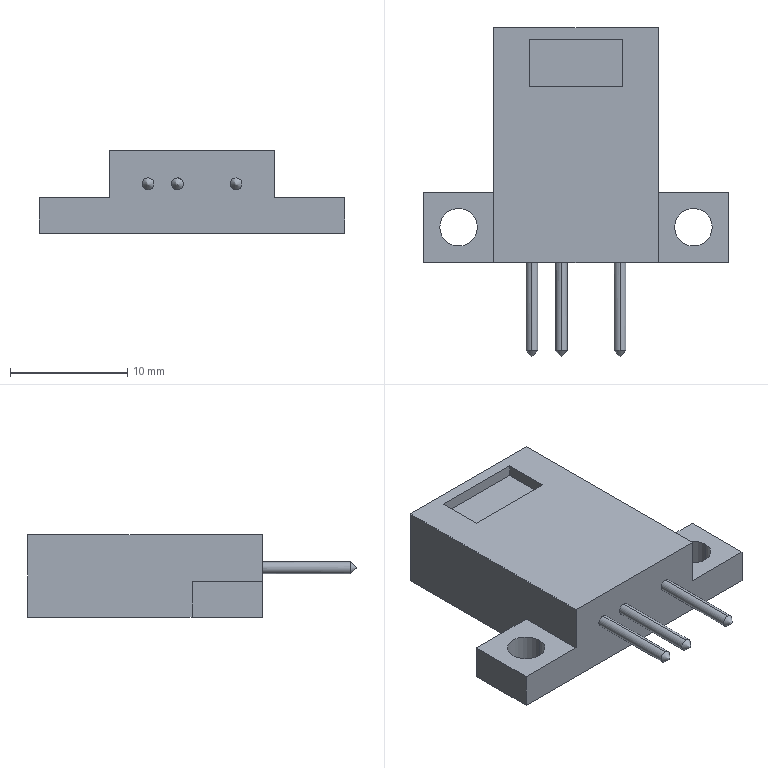Part | SolidWorks | features ICE 4, Dome 1, Extrusion 1 | 1 solid | 30 faces | box 26 x 27.999 x 7 mm | volume 2114 mm3 | plane 17 | cylinder 10 | spline 3 | commonest cylinder face diameters 1 x6 3.2 x4
STEP:
#1=CARTESIAN_POINT('',(3.75,-17.5,3.7));
#2=VERTEX_POINT('',#1);
#3=CARTESIAN_POINT('',(3.75,-17.5,4.7));
#4=VERTEX_POINT('',#3);
#5=CARTESIAN_POINT('',(3.75,-17.5,3.7));
#6=CARTESIAN_POINT('',(3.88,-17.5,3.7));
#7=CARTESIAN_POINT('',(4.011,-17.5,3.754));
#8=CARTESIAN_POINT('',(4.196,-17.5,3.938));
#9=CARTESIAN_POINT('',(4.25,-17.5,4.068));
#10=CARTESIAN_POINT('',(4.25,-17.5,4.332));
#11=CARTESIAN_POINT('',(4.196,-17.5,4.461));
#12=CARTESIAN_POINT('',(4.012,-17.5,4.646));
#13=CARTESIAN_POINT('',(3.882,-17.5,4.7));
#14=CARTESIAN_POINT('',(3.75,-17.5,4.7));
#15=B_SPLINE_CURVE_WITH_KNOTS('',3,(#5,#6,#7,#8,#9,#10,#11,#12,#13,#14),.UNSPECIFIED.,.F.,.F.,(4,2,2,2,4),(0.001565,0.001956,0.002347,0.002738,0.003129),.UNSPECIFIED.);
#16=EDGE_CURVE('',#2,#4,#15,.T.);
#17=ORIENTED_EDGE('',*,*,#16,.F.);
#18=CARTESIAN_POINT('',(3.75,-10.,3.7));
#19=VERTEX_POINT('',#18);
#20=CARTESIAN_POINT('',(3.75,-17.5,3.7));
#21=DIRECTION('',(0.,1.,0.));
#22=VECTOR('',#21,1000.);
#23=LINE('',#20,#22);
#24=EDGE_CURVE('',#2,#19,#23,.T.);
#25=ORIENTED_EDGE('',*,*,#24,.T.);
#26=CARTESIAN_POINT('',(3.75,-10.,4.7));
#27=VERTEX_POINT('',#26);
#28=CARTESIAN_POINT('',(3.75,-10.,4.2));
#29=DIRECTION('',(0.,-1.,0.));
#30=DIRECTION('',(0.,0.,1.));
#31=AXIS2_PLACEMENT_3D('',#28,#29,#30);
#32=CIRCLE('',#31,0.5);
#33=EDGE_CURVE('',#19,#27,#32,.T.);
#34=ORIENTED_EDGE('',*,*,#33,.T.);
#35=CARTESIAN_POINT('',(3.75,-17.5,4.7));
#36=DIRECTION('',(0.,1.,0.));
#37=VECTOR('',#36,1000.);
#38=LINE('',#35,#37);
#39=EDGE_CURVE('',#4,#27,#38,.T.);
#40=ORIENTED_EDGE('',*,*,#39,.F.);
#41=EDGE_LOOP('',(#17,#25,#34,#40));
#42=FACE_OUTER_BOUND('',#41,.T.);
#43=CARTESIAN_POINT('',(3.75,-17.5,4.2));
#44=DIRECTION('',(0.,1.,0.));
#45=DIRECTION('',(0.,0.,1.));
#46=AXIS2_PLACEMENT_3D('',#43,#44,#45);
#47=CYLINDRICAL_SURFACE('',#46,0.5);
#48=ADVANCED_FACE('',(#42),#47,.T.);
#49=CARTESIAN_POINT('',(-1.25,-17.5,3.7));
#50=VERTEX_POINT('',#49);
#51=CARTESIAN_POINT('',(-1.25,-17.5,4.7));
#52=VERTEX_POINT('',#51);
#53=CARTESIAN_POINT('',(-1.25,-17.5,3.7));
#54=CARTESIAN_POINT('',(-1.12,-17.5,3.7));
#55=CARTESIAN_POINT('',(-0.989,-17.5,3.754));
#56=CARTESIAN_POINT('',(-0.8044,-17.5,3.938));
#57=CARTESIAN_POINT('',(-0.7501,-17.5,4.068));
#58=CARTESIAN_POINT('',(-0.7499,-17.5,4.332));
#59=CARTESIAN_POINT('',(-0.804,-17.5,4.461));
#60=CARTESIAN_POINT('',(-0.9884,-17.5,4.646));
#61=CARTESIAN_POINT('',(-1.118,-17.5,4.7));
#62=CARTESIAN_POINT('',(-1.25,-17.5,4.7));
#63=B_SPLINE_CURVE_WITH_KNOTS('',3,(#53,#54,#55,#56,#57,#58,#59,#60,#61,#62),.UNSPECIFIED.,.F.,.F.,(4,2,2,2,4),(0.001565,0.001956,0.002347,0.002738,0.003129),.UNSPECIFIED.);
#64=EDGE_CURVE('',#50,#52,#63,.T.);
#65=ORIENTED_EDGE('',*,*,#64,.F.);
#66=CARTESIAN_POINT('',(-1.25,-10.,3.7));
#67=VERTEX_POINT('',#66);
#68=CARTESIAN_POINT('',(-1.25,-17.5,3.7));
#69=DIRECTION('',(0.,1.,0.));
#70=VECTOR('',#69,1000.);
#71=LINE('',#68,#70);
#72=EDGE_CURVE('',#50,#67,#71,.T.);
#73=ORIENTED_EDGE('',*,*,#72,.T.);
#74=CARTESIAN_POINT('',(-1.25,-10.,4.7));
#75=VERTEX_POINT('',#74);
#76=CARTESIAN_POINT('',(-1.25,-10.,4.2));
#77=DIRECTION('',(0.,-1.,0.));
#78=DIRECTION('',(0.,0.,1.));
#79=AXIS2_PLACEMENT_3D('',#76,#77,#78);
#80=CIRCLE('',#79,0.5);
#81=EDGE_CURVE('',#67,#75,#80,.T.);
#82=ORIENTED_EDGE('',*,*,#81,.T.);
#83=CARTESIAN_POINT('',(-1.25,-17.5,4.7));
#84=DIRECTION('',(0.,1.,0.));
#85=VECTOR('',#84,1000.);
#86=LINE('',#83,#85);
#87=EDGE_CURVE('',#52,#75,#86,.T.);
#88=ORIENTED_EDGE('',*,*,#87,.F.);
#89=EDGE_LOOP('',(#65,#73,#82,#88));
#90=FACE_OUTER_BOUND('',#89,.T.);
#91=CARTESIAN_POINT('',(-1.25,-17.5,4.2));
#92=DIRECTION('',(0.,1.,0.));
#93=DIRECTION('',(0.,0.,1.));
#94=AXIS2_PLACEMENT_3D('',#91,#92,#93);
#95=CYLINDRICAL_SURFACE('',#94,0.5);
#96=ADVANCED_FACE('',(#90),#95,.T.);
#97=CARTESIAN_POINT('',(-3.75,-17.5,3.7));
#98=VERTEX_POINT('',#97);
#99=CARTESIAN_POINT('',(-3.75,-17.5,4.7));
#100=VERTEX_POINT('',#99);
#101=CARTESIAN_POINT('',(-3.75,-17.5,3.7));
#102=CARTESIAN_POINT('',(-3.62,-17.5,3.7));
#103=CARTESIAN_POINT('',(-3.489,-17.5,3.754));
#104=CARTESIAN_POINT('',(-3.304,-17.5,3.938));
#105=CARTESIAN_POINT('',(-3.25,-17.5,4.068));
#106=CARTESIAN_POINT('',(-3.25,-17.5,4.332));
#107=CARTESIAN_POINT('',(-3.304,-17.5,4.461));
#108=CARTESIAN_POINT('',(-3.488,-17.5,4.646));
#109=CARTESIAN_POINT('',(-3.618,-17.5,4.7));
#110=CARTESIAN_POINT('',(-3.75,-17.5,4.7));
#111=B_SPLINE_CURVE_WITH_KNOTS('',3,(#101,#102,#103,#104,#105,#106,#107,#108,#109,#110),.UNSPECIFIED.,.F.,.F.,(4,2,2,2,4),(0.001565,0.001956,0.002347,0.002738,0.003129),.UNSPECIFIED.);
#112=EDGE_CURVE('',#98,#100,#111,.T.);
#113=ORIENTED_EDGE('',*,*,#112,.F.);
#114=CARTESIAN_POINT('',(-3.75,-10.,3.7));
#115=VERTEX_POINT('',#114);
#116=CARTESIAN_POINT('',(-3.75,-17.5,3.7));
#117=DIRECTION('',(0.,1.,0.));
#118=VECTOR('',#117,1000.);
#119=LINE('',#116,#118);
#120=EDGE_CURVE('',#98,#115,#119,.T.);
#121=ORIENTED_EDGE('',*,*,#120,.T.);
#122=CARTESIAN_POINT('',(-3.75,-10.,4.7));
#123=VERTEX_POINT('',#122);
#124=CARTESIAN_POINT('',(-3.75,-10.,4.2));
#125=DIRECTION('',(0.,-1.,0.));
#126=DIRECTION('',(0.,0.,1.));
#127=AXIS2_PLACEMENT_3D('',#124,#125,#126);
#128=CIRCLE('',#127,0.5);
#129=EDGE_CURVE('',#115,#123,#128,.T.);
#130=ORIENTED_EDGE('',*,*,#129,.T.);
#131=CARTESIAN_POINT('',(-3.75,-17.5,4.7));
#132=DIRECTION('',(0.,1.,0.));
#133=VECTOR('',#132,1000.);
#134=LINE('',#131,#133);
#135=EDGE_CURVE('',#100,#123,#134,.T.);
#136=ORIENTED_EDGE('',*,*,#135,.F.);
#137=EDGE_LOOP('',(#113,#121,#130,#136));
#138=FACE_OUTER_BOUND('',#137,.T.);
#139=CARTESIAN_POINT('',(-3.75,-17.5,4.2));
#140=DIRECTION('',(0.,1.,0.));
#141=DIRECTION('',(0.,0.,1.));
#142=AXIS2_PLACEMENT_3D('',#139,#140,#141);
#143=CYLINDRICAL_SURFACE('',#142,0.5);
#144=ADVANCED_FACE('',(#138),#143,.T.);
#145=CARTESIAN_POINT('',(8.4,-7.,0.));
#146=VERTEX_POINT('',#145);
#147=CARTESIAN_POINT('',(11.6,-7.,0.));
#148=VERTEX_POINT('',#147);
#149=CARTESIAN_POINT('',(10.,-7.,0.));
#150=DIRECTION('',(0.,0.,1.));
#151=DIRECTION('',(1.,0.,0.));
#152=AXIS2_PLACEMENT_3D('',#149,#150,#151);
#153=CIRCLE('',#152,1.6);
#154=EDGE_CURVE('',#146,#148,#153,.T.);
#155=ORIENTED_EDGE('',*,*,#154,.F.);
#156=CARTESIAN_POINT('',(8.4,-7.,3.));
#157=VERTEX_POINT('',#156);
#158=CARTESIAN_POINT('',(8.4,-7.,-0.00005));
#159=DIRECTION('',(0.,0.,1.));
#160=VECTOR('',#159,1000.);
#161=LINE('',#158,#160);
#162=EDGE_CURVE('',#146,#157,#161,.T.);
#163=ORIENTED_EDGE('',*,*,#162,.T.);
#164=CARTESIAN_POINT('',(11.6,-7.,3.));
#165=VERTEX_POINT('',#164);
#166=CARTESIAN_POINT('',(10.,-7.,3.));
#167=DIRECTION('',(0.,0.,1.));
#168=DIRECTION('',(-1.,0.,0.));
#169=AXIS2_PLACEMENT_3D('',#166,#167,#168);
#170=CIRCLE('',#169,1.6);
#171=EDGE_CURVE('',#157,#165,#170,.T.);
#172=ORIENTED_EDGE('',*,*,#171,.T.);
#173=CARTESIAN_POINT('',(11.6,-7.,-0.00005));
#174=DIRECTION('',(0.,0.,1.));
#175=VECTOR('',#174,1000.);
#176=LINE('',#173,#175);
#177=EDGE_CURVE('',#148,#165,#176,.T.);
#178=ORIENTED_EDGE('',*,*,#177,.F.);
#179=EDGE_LOOP('',(#155,#163,#172,#178));
#180=FACE_OUTER_BOUND('',#179,.T.);
#181=CARTESIAN_POINT('',(10.,-7.,-0.00005));
#182=DIRECTION('',(0.,0.,1.));
#183=DIRECTION('',(1.,0.,0.));
#184=AXIS2_PLACEMENT_3D('',#181,#182,#183);
#185=CYLINDRICAL_SURFACE('',#184,1.6);
#186=ADVANCED_FACE('',(#180),#185,.F.);
#187=CARTESIAN_POINT('',(-11.6,-7.,0.));
#188=VERTEX_POINT('',#187);
#189=CARTESIAN_POINT('',(-8.4,-7.,0.));
#190=VERTEX_POINT('',#189);
#191=CARTESIAN_POINT('',(-10.,-7.,0.));
#192=DIRECTION('',(0.,0.,1.));
#193=DIRECTION('',(1.,0.,0.));
#194=AXIS2_PLACEMENT_3D('',#191,#192,#193);
#195=CIRCLE('',#194,1.6);
#196=EDGE_CURVE('',#188,#190,#195,.T.);
#197=ORIENTED_EDGE('',*,*,#196,.F.);
#198=CARTESIAN_POINT('',(-11.6,-7.,3.));
#199=VERTEX_POINT('',#198);
#200=CARTESIAN_POINT('',(-11.6,-7.,-0.00005));
#201=DIRECTION('',(0.,0.,1.));
#202=VECTOR('',#201,1000.);
#203=LINE('',#200,#202);
#204=EDGE_CURVE('',#188,#199,#203,.T.);
#205=ORIENTED_EDGE('',*,*,#204,.T.);
#206=CARTESIAN_POINT('',(-8.4,-7.,3.));
#207=VERTEX_POINT('',#206);
#208=CARTESIAN_POINT('',(-10.,-7.,3.));
#209=DIRECTION('',(0.,0.,1.));
#210=DIRECTION('',(1.,0.,0.));
#211=AXIS2_PLACEMENT_3D('',#208,#209,#210);
#212=CIRCLE('',#211,1.6);
#213=EDGE_CURVE('',#199,#207,#212,.T.);
#214=ORIENTED_EDGE('',*,*,#213,.T.);
#215=CARTESIAN_POINT('',(-8.4,-7.,-0.00005));
#216=DIRECTION('',(0.,0.,1.));
#217=VECTOR('',#216,1000.);
#218=LINE('',#215,#217);
#219=EDGE_CURVE('',#190,#207,#218,.T.);
#220=ORIENTED_EDGE('',*,*,#219,.F.);
#221=EDGE_LOOP('',(#197,#205,#214,#220));
#222=FACE_OUTER_BOUND('',#221,.T.);
#223=CARTESIAN_POINT('',(-10.,-7.,-0.00005));
#224=DIRECTION('',(0.,0.,1.));
#225=DIRECTION('',(1.,0.,0.));
#226=AXIS2_PLACEMENT_3D('',#223,#224,#225);
#227=CYLINDRICAL_SURFACE('',#226,1.6);
#228=ADVANCED_FACE('',(#222),#227,.F.);
#229=CARTESIAN_POINT('',(-1.25,-10.,4.2));
#230=DIRECTION('',(0.,-1.,0.));
#231=DIRECTION('',(0.,0.,1.));
#232=AXIS2_PLACEMENT_3D('',#229,#230,#231);
#233=CIRCLE('',#232,0.5);
#234=EDGE_CURVE('',#75,#67,#233,.T.);
#235=ORIENTED_EDGE('',*,*,#234,.F.);
#236=ORIENTED_EDGE('',*,*,#81,.F.);
#237=EDGE_LOOP('',(#235,#236));
#238=FACE_BOUND('',#237,.T.);
#239=CARTESIAN_POINT('',(-13.,-10.,0.));
#240=VERTEX_POINT('',#239);
#241=CARTESIAN_POINT('',(13.,-10.,0.));
#242=VERTEX_POINT('',#241);
#243=CARTESIAN_POINT('',(-7.,-10.,0.));
#244=DIRECTION('',(1.,0.,0.));
#245=VECTOR('',#244,1000.);
#246=LINE('',#243,#245);
#247=EDGE_CURVE('',#240,#242,#246,.T.);
#248=ORIENTED_EDGE('',*,*,#247,.T.);
#249=CARTESIAN_POINT('',(13.,-10.,3.));
#250=VERTEX_POINT('',#249);
#251=CARTESIAN_POINT('',(13.,-10.,3.));
#252=DIRECTION('',(0.,0.,-1.));
#253=VECTOR('',#252,1000.);
#254=LINE('',#251,#253);
#255=EDGE_CURVE('',#250,#242,#254,.T.);
#256=ORIENTED_EDGE('',*,*,#255,.F.);
#257=CARTESIAN_POINT('',(7.,-10.,3.));
#258=VERTEX_POINT('',#257);
#259=CARTESIAN_POINT('',(7.,-10.,3.));
#260=DIRECTION('',(-1.,0.,0.));
#261=VECTOR('',#260,1000.);
#262=LINE('',#259,#261);
#263=EDGE_CURVE('',#250,#258,#262,.T.);
#264=ORIENTED_EDGE('',*,*,#263,.T.);
#265=CARTESIAN_POINT('',(7.,-10.,7.));
#266=VERTEX_POINT('',#265);
#267=CARTESIAN_POINT('',(7.,-10.,7.));
#268=DIRECTION('',(0.,0.,-1.));
#269=VECTOR('',#268,1000.);
#270=LINE('',#267,#269);
#271=EDGE_CURVE('',#266,#258,#270,.T.);
#272=ORIENTED_EDGE('',*,*,#271,.F.);
#273=CARTESIAN_POINT('',(-7.,-10.,7.));
#274=VERTEX_POINT('',#273);
#275=CARTESIAN_POINT('',(-7.,-10.,7.));
#276=DIRECTION('',(1.,0.,0.));
#277=VECTOR('',#276,1000.);
#278=LINE('',#275,#277);
#279=EDGE_CURVE('',#274,#266,#278,.T.);
#280=ORIENTED_EDGE('',*,*,#279,.F.);
#281=CARTESIAN_POINT('',(-7.,-10.,3.));
#282=VERTEX_POINT('',#281);
#283=CARTESIAN_POINT('',(-7.,-10.,7.));
#284=DIRECTION('',(0.,0.,-1.));
#285=VECTOR('',#284,1000.);
#286=LINE('',#283,#285);
#287=EDGE_CURVE('',#274,#282,#286,.T.);
#288=ORIENTED_EDGE('',*,*,#287,.T.);
#289=CARTESIAN_POINT('',(-13.,-10.,3.));
#290=VERTEX_POINT('',#289);
#291=CARTESIAN_POINT('',(-7.,-10.,3.));
#292=DIRECTION('',(-1.,0.,0.));
#293=VECTOR('',#292,1000.);
#294=LINE('',#291,#293);
#295=EDGE_CURVE('',#282,#290,#294,.T.);
#296=ORIENTED_EDGE('',*,*,#295,.T.);
#297=CARTESIAN_POINT('',(-13.,-10.,3.));
#298=DIRECTION('',(0.,0.,-1.));
#299=VECTOR('',#298,1000.);
#300=LINE('',#297,#299);
#301=EDGE_CURVE('',#290,#240,#300,.T.);
#302=ORIENTED_EDGE('',*,*,#301,.T.);
#303=EDGE_LOOP('',(#248,#256,#264,#272,#280,#288,#296,#302));
#304=FACE_OUTER_BOUND('',#303,.T.);
#305=CARTESIAN_POINT('',(-3.75,-10.,4.2));
#306=DIRECTION('',(0.,-1.,0.));
#307=DIRECTION('',(0.,0.,1.));
#308=AXIS2_PLACEMENT_3D('',#305,#306,#307);
#309=CIRCLE('',#308,0.5);
#310=EDGE_CURVE('',#123,#115,#309,.T.);
#311=ORIENTED_EDGE('',*,*,#310,.F.);
#312=ORIENTED_EDGE('',*,*,#129,.F.);
#313=EDGE_LOOP('',(#311,#312));
#314=FACE_BOUND('',#313,.T.);
#315=CARTESIAN_POINT('',(3.75,-10.,4.2));
#316=DIRECTION('',(0.,-1.,0.));
#317=DIRECTION('',(0.,0.,1.));
#318=AXIS2_PLACEMENT_3D('',#315,#316,#317);
#319=CIRCLE('',#318,0.5);
#320=EDGE_CURVE('',#27,#19,#319,.T.);
#321=ORIENTED_EDGE('',*,*,#320,.F.);
#322=ORIENTED_EDGE('',*,*,#33,.F.);
#323=EDGE_LOOP('',(#321,#322));
#324=FACE_BOUND('',#323,.T.);
#325=CARTESIAN_POINT('',(-7.,-10.,7.));
#326=DIRECTION('',(0.,1.,0.));
#327=DIRECTION('',(0.,0.,1.));
#328=AXIS2_PLACEMENT_3D('',#325,#326,#327);
#329=PLANE('',#328);
#330=ADVANCED_FACE('',(#238,#304,#314,#324),#329,.F.);
#331=CARTESIAN_POINT('',(-7.,-4.,3.));
#332=VERTEX_POINT('',#331);
#333=CARTESIAN_POINT('',(-7.,-4.,0.));
#334=VERTEX_POINT('',#333);
#335=CARTESIAN_POINT('',(-7.,-4.,3.));
#336=DIRECTION('',(0.,0.,-1.));
#337=VECTOR('',#336,1000.);
#338=LINE('',#335,#337);
#339=EDGE_CURVE('',#332,#334,#338,.T.);
#340=ORIENTED_EDGE('',*,*,#339,.F.);
#341=CARTESIAN_POINT('',(-7.,-4.,3.));
#342=DIRECTION('',(0.,-1.,0.));
#343=VECTOR('',#342,1000.);
#344=LINE('',#341,#343);
#345=EDGE_CURVE('',#332,#282,#344,.T.);
#346=ORIENTED_EDGE('',*,*,#345,.T.);
#347=ORIENTED_EDGE('',*,*,#287,.F.);
#348=CARTESIAN_POINT('',(-7.,10.,7.));
#349=VERTEX_POINT('',#348);
#350=CARTESIAN_POINT('',(-7.,10.,7.));
#351=DIRECTION('',(0.,-1.,0.));
#352=VECTOR('',#351,1000.);
#353=LINE('',#350,#352);
#354=EDGE_CURVE('',#349,#274,#353,.T.);
#355=ORIENTED_EDGE('',*,*,#354,.F.);
#356=CARTESIAN_POINT('',(-7.,10.,0.));
#357=VERTEX_POINT('',#356);
#358=CARTESIAN_POINT('',(-7.,10.,7.));
#359=DIRECTION('',(0.,0.,-1.));
#360=VECTOR('',#359,1000.);
#361=LINE('',#358,#360);
#362=EDGE_CURVE('',#349,#357,#361,.T.);
#363=ORIENTED_EDGE('',*,*,#362,.T.);
#364=CARTESIAN_POINT('',(-7.,10.,0.));
#365=DIRECTION('',(0.,-1.,0.));
#366=VECTOR('',#365,1000.);
#367=LINE('',#364,#366);
#368=EDGE_CURVE('',#357,#334,#367,.T.);
#369=ORIENTED_EDGE('',*,*,#368,.T.);
#370=EDGE_LOOP('',(#340,#346,#347,#355,#363,#369));
#371=FACE_OUTER_BOUND('',#370,.T.);
#372=CARTESIAN_POINT('',(-7.,10.,7.));
#373=DIRECTION('',(1.,0.,0.));
#374=DIRECTION('',(0.,1.,0.));
#375=AXIS2_PLACEMENT_3D('',#372,#373,#374);
#376=PLANE('',#375);
#377=ADVANCED_FACE('',(#371),#376,.F.);
#378=ORIENTED_EDGE('',*,*,#271,.T.);
#379=CARTESIAN_POINT('',(7.,-4.,3.));
#380=VERTEX_POINT('',#379);
#381=CARTESIAN_POINT('',(7.,-4.,3.));
#382=DIRECTION('',(0.,1.,0.));
#383=VECTOR('',#382,1000.);
#384=LINE('',#381,#383);
#385=EDGE_CURVE('',#258,#380,#384,.T.);
#386=ORIENTED_EDGE('',*,*,#385,.T.);
#387=CARTESIAN_POINT('',(7.,-4.,0.));
#388=VERTEX_POINT('',#387);
#389=CARTESIAN_POINT('',(7.,-4.,3.));
#390=DIRECTION('',(0.,0.,-1.));
#391=VECTOR('',#390,1000.);
#392=LINE('',#389,#391);
#393=EDGE_CURVE('',#380,#388,#392,.T.);
#394=ORIENTED_EDGE('',*,*,#393,.T.);
#395=CARTESIAN_POINT('',(7.,10.,0.));
#396=VERTEX_POINT('',#395);
#397=CARTESIAN_POINT('',(7.,10.,0.));
#398=DIRECTION('',(0.,1.,0.));
#399=VECTOR('',#398,1000.);
#400=LINE('',#397,#399);
#401=EDGE_CURVE('',#388,#396,#400,.T.);
#402=ORIENTED_EDGE('',*,*,#401,.T.);
#403=CARTESIAN_POINT('',(7.,10.,7.));
#404=VERTEX_POINT('',#403);
#405=CARTESIAN_POINT('',(7.,10.,7.));
#406=DIRECTION('',(0.,0.,-1.));
#407=VECTOR('',#406,1000.);
#408=LINE('',#405,#407);
#409=EDGE_CURVE('',#404,#396,#408,.T.);
#410=ORIENTED_EDGE('',*,*,#409,.F.);
#411=CARTESIAN_POINT('',(7.,10.,7.));
#412=DIRECTION('',(0.,1.,0.));
#413=VECTOR('',#412,1000.);
#414=LINE('',#411,#413);
#415=EDGE_CURVE('',#266,#404,#414,.T.);
#416=ORIENTED_EDGE('',*,*,#415,.F.);
#417=EDGE_LOOP('',(#378,#386,#394,#402,#410,#416));
#418=FACE_OUTER_BOUND('',#417,.T.);
#419=CARTESIAN_POINT('',(7.,10.,7.));
#420=DIRECTION('',(-1.,0.,0.));
#421=DIRECTION('',(0.,-1.,0.));
#422=AXIS2_PLACEMENT_3D('',#419,#420,#421);
#423=PLANE('',#422);
#424=ADVANCED_FACE('',(#418),#423,.F.);
#425=CARTESIAN_POINT('',(-7.,10.,0.));
#426=DIRECTION('',(-1.,0.,0.));
#427=VECTOR('',#426,1000.);
#428=LINE('',#425,#427);
#429=EDGE_CURVE('',#396,#357,#428,.T.);
#430=ORIENTED_EDGE('',*,*,#429,.T.);
#431=ORIENTED_EDGE('',*,*,#362,.F.);
#432=CARTESIAN_POINT('',(-7.,10.,7.));
#433=DIRECTION('',(-1.,0.,0.));
#434=VECTOR('',#433,1000.);
#435=LINE('',#432,#434);
#436=EDGE_CURVE('',#404,#349,#435,.T.);
#437=ORIENTED_EDGE('',*,*,#436,.F.);
#438=ORIENTED_EDGE('',*,*,#409,.T.);
#439=EDGE_LOOP('',(#430,#431,#437,#438));
#440=FACE_OUTER_BOUND('',#439,.T.);
#441=CARTESIAN_POINT('',(-7.,10.,7.));
#442=DIRECTION('',(0.,-1.,0.));
#443=DIRECTION('',(0.,0.,-1.));
#444=AXIS2_PLACEMENT_3D('',#441,#442,#443);
#445=PLANE('',#444);
#446=ADVANCED_FACE('',(#440),#445,.F.);
#447=CARTESIAN_POINT('',(-4.,9.,7.));
#448=VERTEX_POINT('',#447);
#449=CARTESIAN_POINT('',(-4.,5.,7.));
#450=VERTEX_POINT('',#449);
#451=CARTESIAN_POINT('',(-4.,9.,7.));
#452=DIRECTION('',(0.,-1.,0.));
#453=VECTOR('',#452,1000.);
#454=LINE('',#451,#453);
#455=EDGE_CURVE('',#448,#450,#454,.T.);
#456=ORIENTED_EDGE('',*,*,#455,.F.);
#457=CARTESIAN_POINT('',(4.,9.,7.));
#458=VERTEX_POINT('',#457);
#459=CARTESIAN_POINT('',(-4.,9.,7.));
#460=DIRECTION('',(-1.,0.,0.));
#461=VECTOR('',#460,1000.);
#462=LINE('',#459,#461);
#463=EDGE_CURVE('',#458,#448,#462,.T.);
#464=ORIENTED_EDGE('',*,*,#463,.F.);
#465=CARTESIAN_POINT('',(4.,5.,7.));
#466=VERTEX_POINT('',#465);
#467=CARTESIAN_POINT('',(4.,9.,7.));
#468=DIRECTION('',(0.,1.,0.));
#469=VECTOR('',#468,1000.);
#470=LINE('',#467,#469);
#471=EDGE_CURVE('',#466,#458,#470,.T.);
#472=ORIENTED_EDGE('',*,*,#471,.F.);
#473=CARTESIAN_POINT('',(-4.,5.,7.));
#474=DIRECTION('',(1.,0.,0.));
#475=VECTOR('',#474,1000.);
#476=LINE('',#473,#475);
#477=EDGE_CURVE('',#450,#466,#476,.T.);
#478=ORIENTED_EDGE('',*,*,#477,.F.);
#479=EDGE_LOOP('',(#456,#464,#472,#478));
#480=FACE_BOUND('',#479,.T.);
#481=ORIENTED_EDGE('',*,*,#354,.T.);
#482=ORIENTED_EDGE('',*,*,#279,.T.);
#483=ORIENTED_EDGE('',*,*,#415,.T.);
#484=ORIENTED_EDGE('',*,*,#436,.T.);
#485=EDGE_LOOP('',(#481,#482,#483,#484));
#486=FACE_OUTER_BOUND('',#485,.T.);
#487=CARTESIAN_POINT('',(-7.,-10.,7.));
#488=DIRECTION('',(0.,0.,1.));
#489=DIRECTION('',(1.,0.,0.));
#490=AXIS2_PLACEMENT_3D('',#487,#488,#489);
#491=PLANE('',#490);
#492=ADVANCED_FACE('',(#480,#486),#491,.T.);
#493=CARTESIAN_POINT('',(10.,-7.,0.));
#494=DIRECTION('',(0.,0.,1.));
#495=DIRECTION('',(1.,0.,0.));
#496=AXIS2_PLACEMENT_3D('',#493,#494,#495);
#497=CIRCLE('',#496,1.6);
#498=EDGE_CURVE('',#148,#146,#497,.T.);
#499=ORIENTED_EDGE('',*,*,#498,.T.);
#500=ORIENTED_EDGE('',*,*,#154,.T.);
#501=EDGE_LOOP('',(#499,#500));
#502=FACE_BOUND('',#501,.T.);
#503=CARTESIAN_POINT('',(-10.,-7.,0.));
#504=DIRECTION('',(0.,0.,1.));
#505=DIRECTION('',(1.,0.,0.));
#506=AXIS2_PLACEMENT_3D('',#503,#504,#505);
#507=CIRCLE('',#506,1.6);
#508=EDGE_CURVE('',#190,#188,#507,.T.);
#509=ORIENTED_EDGE('',*,*,#508,.T.);
#510=ORIENTED_EDGE('',*,*,#196,.T.);
#511=EDGE_LOOP('',(#509,#510));
#512=FACE_BOUND('',#511,.T.);
#513=ORIENTED_EDGE('',*,*,#368,.F.);
#514=ORIENTED_EDGE('',*,*,#429,.F.);
#515=ORIENTED_EDGE('',*,*,#401,.F.);
#516=CARTESIAN_POINT('',(13.,-4.,0.));
#517=VERTEX_POINT('',#516);
#518=CARTESIAN_POINT('',(7.,-4.,0.));
#519=DIRECTION('',(1.,0.,0.));
#520=VECTOR('',#519,1000.);
#521=LINE('',#518,#520);
#522=EDGE_CURVE('',#388,#517,#521,.T.);
#523=ORIENTED_EDGE('',*,*,#522,.T.);
#524=CARTESIAN_POINT('',(13.,-4.,0.));
#525=DIRECTION('',(0.,-1.,0.));
#526=VECTOR('',#525,1000.);
#527=LINE('',#524,#526);
#528=EDGE_CURVE('',#517,#242,#527,.T.);
#529=ORIENTED_EDGE('',*,*,#528,.T.);
#530=ORIENTED_EDGE('',*,*,#247,.F.);
#531=CARTESIAN_POINT('',(-13.,-4.,0.));
#532=VERTEX_POINT('',#531);
#533=CARTESIAN_POINT('',(-13.,-4.,0.));
#534=DIRECTION('',(0.,1.,0.));
#535=VECTOR('',#534,1000.);
#536=LINE('',#533,#535);
#537=EDGE_CURVE('',#240,#532,#536,.T.);
#538=ORIENTED_EDGE('',*,*,#537,.T.);
#539=CARTESIAN_POINT('',(-7.,-4.,0.));
#540=DIRECTION('',(1.,0.,0.));
#541=VECTOR('',#540,1000.);
#542=LINE('',#539,#541);
#543=EDGE_CURVE('',#532,#334,#542,.T.);
#544=ORIENTED_EDGE('',*,*,#543,.T.);
#545=EDGE_LOOP('',(#513,#514,#515,#523,#529,#530,#538,#544));
#546=FACE_OUTER_BOUND('',#545,.T.);
#547=CARTESIAN_POINT('',(-7.,-10.,0.));
#548=DIRECTION('',(0.,0.,1.));
#549=DIRECTION('',(1.,0.,0.));
#550=AXIS2_PLACEMENT_3D('',#547,#548,#549);
#551=PLANE('',#550);
#552=ADVANCED_FACE('',(#502,#512,#546),#551,.F.);
#553=ORIENTED_EDGE('',*,*,#528,.F.);
#554=CARTESIAN_POINT('',(13.,-4.,3.));
#555=VERTEX_POINT('',#554);
#556=CARTESIAN_POINT('',(13.,-4.,3.));
#557=DIRECTION('',(0.,0.,-1.));
#558=VECTOR('',#557,1000.);
#559=LINE('',#556,#558);
#560=EDGE_CURVE('',#555,#517,#559,.T.);
#561=ORIENTED_EDGE('',*,*,#560,.F.);
#562=CARTESIAN_POINT('',(13.,-4.,3.));
#563=DIRECTION('',(0.,-1.,0.));
#564=VECTOR('',#563,1000.);
#565=LINE('',#562,#564);
#566=EDGE_CURVE('',#555,#250,#565,.T.);
#567=ORIENTED_EDGE('',*,*,#566,.T.);
#568=ORIENTED_EDGE('',*,*,#255,.T.);
#569=EDGE_LOOP('',(#553,#561,#567,#568));
#570=FACE_OUTER_BOUND('',#569,.T.);
#571=CARTESIAN_POINT('',(13.,-4.,3.));
#572=DIRECTION('',(1.,0.,0.));
#573=DIRECTION('',(0.,1.,0.));
#574=AXIS2_PLACEMENT_3D('',#571,#572,#573);
#575=PLANE('',#574);
#576=ADVANCED_FACE('',(#570),#575,.T.);
#577=ORIENTED_EDGE('',*,*,#522,.F.);
#578=ORIENTED_EDGE('',*,*,#393,.F.);
#579=CARTESIAN_POINT('',(7.,-4.,3.));
#580=DIRECTION('',(1.,0.,0.));
#581=VECTOR('',#580,1000.);
#582=LINE('',#579,#581);
#583=EDGE_CURVE('',#380,#555,#582,.T.);
#584=ORIENTED_EDGE('',*,*,#583,.T.);
#585=ORIENTED_EDGE('',*,*,#560,.T.);
#586=EDGE_LOOP('',(#577,#578,#584,#585));
#587=FACE_OUTER_BOUND('',#586,.T.);
#588=CARTESIAN_POINT('',(7.,-4.,3.));
#589=DIRECTION('',(0.,1.,0.));
#590=DIRECTION('',(-1.,0.,0.));
#591=AXIS2_PLACEMENT_3D('',#588,#589,#590);
#592=PLANE('',#591);
#593=ADVANCED_FACE('',(#587),#592,.T.);
#594=CARTESIAN_POINT('',(10.,-7.,3.));
#595=DIRECTION('',(0.,0.,1.));
#596=DIRECTION('',(-1.,0.,0.));
#597=AXIS2_PLACEMENT_3D('',#594,#595,#596);
#598=CIRCLE('',#597,1.6);
#599=EDGE_CURVE('',#165,#157,#598,.T.);
#600=ORIENTED_EDGE('',*,*,#599,.F.);
#601=ORIENTED_EDGE('',*,*,#171,.F.);
#602=EDGE_LOOP('',(#600,#601));
#603=FACE_BOUND('',#602,.T.);
#604=ORIENTED_EDGE('',*,*,#385,.F.);
#605=ORIENTED_EDGE('',*,*,#263,.F.);
#606=ORIENTED_EDGE('',*,*,#566,.F.);
#607=ORIENTED_EDGE('',*,*,#583,.F.);
#608=EDGE_LOOP('',(#604,#605,#606,#607));
#609=FACE_OUTER_BOUND('',#608,.T.);
#610=CARTESIAN_POINT('',(7.,-10.,3.));
#611=DIRECTION('',(0.,0.,1.));
#612=DIRECTION('',(1.,0.,0.));
#613=AXIS2_PLACEMENT_3D('',#610,#611,#612);
#614=PLANE('',#613);
#615=ADVANCED_FACE('',(#603,#609),#614,.T.);
#616=ORIENTED_EDGE('',*,*,#543,.F.);
#617=CARTESIAN_POINT('',(-13.,-4.,3.));
#618=VERTEX_POINT('',#617);
#619=CARTESIAN_POINT('',(-13.,-4.,3.));
#620=DIRECTION('',(0.,0.,-1.));
#621=VECTOR('',#620,1000.);
#622=LINE('',#619,#621);
#623=EDGE_CURVE('',#618,#532,#622,.T.);
#624=ORIENTED_EDGE('',*,*,#623,.F.);
#625=CARTESIAN_POINT('',(-7.,-4.,3.));
#626=DIRECTION('',(1.,0.,0.));
#627=VECTOR('',#626,1000.);
#628=LINE('',#625,#627);
#629=EDGE_CURVE('',#618,#332,#628,.T.);
#630=ORIENTED_EDGE('',*,*,#629,.T.);
#631=ORIENTED_EDGE('',*,*,#339,.T.);
#632=EDGE_LOOP('',(#616,#624,#630,#631));
#633=FACE_OUTER_BOUND('',#632,.T.);
#634=CARTESIAN_POINT('',(-7.,-4.,3.));
#635=DIRECTION('',(0.,1.,0.));
#636=DIRECTION('',(-1.,0.,0.));
#637=AXIS2_PLACEMENT_3D('',#634,#635,#636);
#638=PLANE('',#637);
#639=ADVANCED_FACE('',(#633),#638,.T.);
#640=ORIENTED_EDGE('',*,*,#537,.F.);
#641=ORIENTED_EDGE('',*,*,#301,.F.);
#642=CARTESIAN_POINT('',(-13.,-4.,3.));
#643=DIRECTION('',(0.,1.,0.));
#644=VECTOR('',#643,1000.);
#645=LINE('',#642,#644);
#646=EDGE_CURVE('',#290,#618,#645,.T.);
#647=ORIENTED_EDGE('',*,*,#646,.T.);
#648=ORIENTED_EDGE('',*,*,#623,.T.);
#649=EDGE_LOOP('',(#640,#641,#647,#648));
#650=FACE_OUTER_BOUND('',#649,.T.);
#651=CARTESIAN_POINT('',(-13.,-4.,3.));
#652=DIRECTION('',(-1.,0.,0.));
#653=DIRECTION('',(0.,0.,1.));
#654=AXIS2_PLACEMENT_3D('',#651,#652,#653);
#655=PLANE('',#654);
#656=ADVANCED_FACE('',(#650),#655,.T.);
#657=CARTESIAN_POINT('',(-10.,-7.,3.));
#658=DIRECTION('',(0.,0.,1.));
#659=DIRECTION('',(1.,0.,0.));
#660=AXIS2_PLACEMENT_3D('',#657,#658,#659);
#661=CIRCLE('',#660,1.6);
#662=EDGE_CURVE('',#207,#199,#661,.T.);
#663=ORIENTED_EDGE('',*,*,#662,.F.);
#664=ORIENTED_EDGE('',*,*,#213,.F.);
#665=EDGE_LOOP('',(#663,#664));
#666=FACE_BOUND('',#665,.T.);
#667=ORIENTED_EDGE('',*,*,#629,.F.);
#668=ORIENTED_EDGE('',*,*,#646,.F.);
#669=ORIENTED_EDGE('',*,*,#295,.F.);
#670=ORIENTED_EDGE('',*,*,#345,.F.);
#671=EDGE_LOOP('',(#667,#668,#669,#670));
#672=FACE_OUTER_BOUND('',#671,.T.);
#673=CARTESIAN_POINT('',(-13.,-4.,3.));
#674=DIRECTION('',(0.,0.,1.));
#675=DIRECTION('',(1.,0.,0.));
#676=AXIS2_PLACEMENT_3D('',#673,#674,#675);
#677=PLANE('',#676);
#678=ADVANCED_FACE('',(#666,#672),#677,.T.);
#679=ORIENTED_EDGE('',*,*,#204,.F.);
#680=ORIENTED_EDGE('',*,*,#508,.F.);
#681=ORIENTED_EDGE('',*,*,#219,.T.);
#682=ORIENTED_EDGE('',*,*,#662,.T.);
#683=EDGE_LOOP('',(#679,#680,#681,#682));
#684=FACE_OUTER_BOUND('',#683,.T.);
#685=CARTESIAN_POINT('',(-10.,-7.,-0.00005));
#686=DIRECTION('',(0.,0.,1.));
#687=DIRECTION('',(1.,0.,0.));
#688=AXIS2_PLACEMENT_3D('',#685,#686,#687);
#689=CYLINDRICAL_SURFACE('',#688,1.6);
#690=ADVANCED_FACE('',(#684),#689,.F.);
#691=ORIENTED_EDGE('',*,*,#162,.F.);
#692=ORIENTED_EDGE('',*,*,#498,.F.);
#693=ORIENTED_EDGE('',*,*,#177,.T.);
#694=ORIENTED_EDGE('',*,*,#599,.T.);
#695=EDGE_LOOP('',(#691,#692,#693,#694));
#696=FACE_OUTER_BOUND('',#695,.T.);
#697=CARTESIAN_POINT('',(10.,-7.,-0.00005));
#698=DIRECTION('',(0.,0.,1.));
#699=DIRECTION('',(1.,0.,0.));
#700=AXIS2_PLACEMENT_3D('',#697,#698,#699);
#701=CYLINDRICAL_SURFACE('',#700,1.6);
#702=ADVANCED_FACE('',(#696),#701,.F.);
#703=ORIENTED_EDGE('',*,*,#455,.T.);
#704=CARTESIAN_POINT('',(-4.,5.,6.));
#705=VERTEX_POINT('',#704);
#706=CARTESIAN_POINT('',(-4.,5.,6.));
#707=DIRECTION('',(0.,0.,1.));
#708=VECTOR('',#707,1000.);
#709=LINE('',#706,#708);
#710=EDGE_CURVE('',#705,#450,#709,.T.);
#711=ORIENTED_EDGE('',*,*,#710,.F.);
#712=CARTESIAN_POINT('',(-4.,9.,6.));
#713=VERTEX_POINT('',#712);
#714=CARTESIAN_POINT('',(-4.,9.,6.));
#715=DIRECTION('',(0.,-1.,0.));
#716=VECTOR('',#715,1000.);
#717=LINE('',#714,#716);
#718=EDGE_CURVE('',#713,#705,#717,.T.);
#719=ORIENTED_EDGE('',*,*,#718,.F.);
#720=CARTESIAN_POINT('',(-4.,9.,6.));
#721=DIRECTION('',(0.,0.,1.));
#722=VECTOR('',#721,1000.);
#723=LINE('',#720,#722);
#724=EDGE_CURVE('',#713,#448,#723,.T.);
#725=ORIENTED_EDGE('',*,*,#724,.T.);
#726=EDGE_LOOP('',(#703,#711,#719,#725));
#727=FACE_OUTER_BOUND('',#726,.T.);
#728=CARTESIAN_POINT('',(-4.,9.,6.));
#729=DIRECTION('',(-1.,0.,0.));
#730=DIRECTION('',(0.,-1.,0.));
#731=AXIS2_PLACEMENT_3D('',#728,#729,#730);
#732=PLANE('',#731);
#733=ADVANCED_FACE('',(#727),#732,.F.);
#734=ORIENTED_EDGE('',*,*,#463,.T.);
#735=ORIENTED_EDGE('',*,*,#724,.F.);
#736=CARTESIAN_POINT('',(4.,9.,6.));
#737=VERTEX_POINT('',#736);
#738=CARTESIAN_POINT('',(-4.,9.,6.));
#739=DIRECTION('',(-1.,0.,0.));
#740=VECTOR('',#739,1000.);
#741=LINE('',#738,#740);
#742=EDGE_CURVE('',#737,#713,#741,.T.);
#743=ORIENTED_EDGE('',*,*,#742,.F.);
#744=CARTESIAN_POINT('',(4.,9.,6.));
#745=DIRECTION('',(0.,0.,1.));
#746=VECTOR('',#745,1000.);
#747=LINE('',#744,#746);
#748=EDGE_CURVE('',#737,#458,#747,.T.);
#749=ORIENTED_EDGE('',*,*,#748,.T.);
#750=EDGE_LOOP('',(#734,#735,#743,#749));
#751=FACE_OUTER_BOUND('',#750,.T.);
#752=CARTESIAN_POINT('',(-4.,9.,6.));
#753=DIRECTION('',(0.,1.,0.));
#754=DIRECTION('',(0.,0.,1.));
#755=AXIS2_PLACEMENT_3D('',#752,#753,#754);
#756=PLANE('',#755);
#757=ADVANCED_FACE('',(#751),#756,.F.);
#758=ORIENTED_EDGE('',*,*,#471,.T.);
#759=ORIENTED_EDGE('',*,*,#748,.F.);
#760=CARTESIAN_POINT('',(4.,5.,6.));
#761=VERTEX_POINT('',#760);
#762=CARTESIAN_POINT('',(4.,9.,6.));
#763=DIRECTION('',(0.,1.,0.));
#764=VECTOR('',#763,1000.);
#765=LINE('',#762,#764);
#766=EDGE_CURVE('',#761,#737,#765,.T.);
#767=ORIENTED_EDGE('',*,*,#766,.F.);
#768=CARTESIAN_POINT('',(4.,5.,6.));
#769=DIRECTION('',(0.,0.,1.));
#770=VECTOR('',#769,1000.);
#771=LINE('',#768,#770);
#772=EDGE_CURVE('',#761,#466,#771,.T.);
#773=ORIENTED_EDGE('',*,*,#772,.T.);
#774=EDGE_LOOP('',(#758,#759,#767,#773));
#775=FACE_OUTER_BOUND('',#774,.T.);
#776=CARTESIAN_POINT('',(4.,9.,6.));
#777=DIRECTION('',(1.,0.,0.));
#778=DIRECTION('',(0.,1.,0.));
#779=AXIS2_PLACEMENT_3D('',#776,#777,#778);
#780=PLANE('',#779);
#781=ADVANCED_FACE('',(#775),#780,.F.);
#782=ORIENTED_EDGE('',*,*,#477,.T.);
#783=ORIENTED_EDGE('',*,*,#772,.F.);
#784=CARTESIAN_POINT('',(-4.,5.,6.));
#785=DIRECTION('',(1.,0.,0.));
#786=VECTOR('',#785,1000.);
#787=LINE('',#784,#786);
#788=EDGE_CURVE('',#705,#761,#787,.T.);
#789=ORIENTED_EDGE('',*,*,#788,.F.);
#790=ORIENTED_EDGE('',*,*,#710,.T.);
#791=EDGE_LOOP('',(#782,#783,#789,#790));
#792=FACE_OUTER_BOUND('',#791,.T.);
#793=CARTESIAN_POINT('',(-4.,5.,6.));
#794=DIRECTION('',(0.,-1.,0.));
#795=DIRECTION('',(0.,0.,-1.));
#796=AXIS2_PLACEMENT_3D('',#793,#794,#795);
#797=PLANE('',#796);
#798=ADVANCED_FACE('',(#792),#797,.F.);
#799=ORIENTED_EDGE('',*,*,#718,.T.);
#800=ORIENTED_EDGE('',*,*,#788,.T.);
#801=ORIENTED_EDGE('',*,*,#766,.T.);
#802=ORIENTED_EDGE('',*,*,#742,.T.);
#803=EDGE_LOOP('',(#799,#800,#801,#802));
#804=FACE_OUTER_BOUND('',#803,.T.);
#805=CARTESIAN_POINT('',(-4.,5.,6.));
#806=DIRECTION('',(0.,0.,1.));
#807=DIRECTION('',(1.,0.,0.));
#808=AXIS2_PLACEMENT_3D('',#805,#806,#807);
#809=PLANE('',#808);
#810=ADVANCED_FACE('',(#804),#809,.T.);
#811=ORIENTED_EDGE('',*,*,#120,.F.);
#812=CARTESIAN_POINT('',(-3.75,-17.5,4.7));
#813=CARTESIAN_POINT('',(-3.882,-17.5,4.7));
#814=CARTESIAN_POINT('',(-4.011,-17.5,4.646));
#815=CARTESIAN_POINT('',(-4.196,-17.5,4.461));
#816=CARTESIAN_POINT('',(-4.25,-17.5,4.331));
#817=CARTESIAN_POINT('',(-4.25,-17.5,4.07));
#818=CARTESIAN_POINT('',(-4.197,-17.5,3.94));
#819=CARTESIAN_POINT('',(-4.01,-17.5,3.753));
#820=CARTESIAN_POINT('',(-3.88,-17.5,3.7));
#821=CARTESIAN_POINT('',(-3.75,-17.5,3.7));
#822=B_SPLINE_CURVE_WITH_KNOTS('',3,(#812,#813,#814,#815,#816,#817,#818,#819,#820,#821),.UNSPECIFIED.,.F.,.F.,(4,2,2,2,4),(0.,0.0003911,0.0007823,0.001173,0.001565),.UNSPECIFIED.);
#823=EDGE_CURVE('',#100,#98,#822,.T.);
#824=ORIENTED_EDGE('',*,*,#823,.F.);
#825=ORIENTED_EDGE('',*,*,#135,.T.);
#826=ORIENTED_EDGE('',*,*,#310,.T.);
#827=EDGE_LOOP('',(#811,#824,#825,#826));
#828=FACE_OUTER_BOUND('',#827,.T.);
#829=CARTESIAN_POINT('',(-3.75,-17.5,4.2));
#830=DIRECTION('',(0.,1.,0.));
#831=DIRECTION('',(0.,0.,1.));
#832=AXIS2_PLACEMENT_3D('',#829,#830,#831);
#833=CYLINDRICAL_SURFACE('',#832,0.5);
#834=ADVANCED_FACE('',(#828),#833,.T.);
#835=ORIENTED_EDGE('',*,*,#823,.T.);
#836=ORIENTED_EDGE('',*,*,#112,.T.);
#837=EDGE_LOOP('',(#835,#836));
#838=FACE_OUTER_BOUND('',#837,.T.);
#839=CARTESIAN_POINT('',(-3.234,-17.204,3.685));
#840=CARTESIAN_POINT('',(-3.234,-17.273,3.767));
#841=CARTESIAN_POINT('',(-3.234,-17.336,3.85));
#842=CARTESIAN_POINT('',(-3.234,-17.395,3.932));
#843=CARTESIAN_POINT('',(-3.234,-17.461,4.056));
#844=CARTESIAN_POINT('',(-3.234,-17.479,4.179));
#845=CARTESIAN_POINT('',(-3.234,-17.479,4.221));
#846=CARTESIAN_POINT('',(-3.234,-17.461,4.344));
#847=CARTESIAN_POINT('',(-3.234,-17.395,4.468));
#848=CARTESIAN_POINT('',(-3.234,-17.336,4.55));
#849=CARTESIAN_POINT('',(-3.234,-17.273,4.633));
#850=CARTESIAN_POINT('',(-3.234,-17.204,4.715));
#851=CARTESIAN_POINT('',(-3.316,-17.274,3.685));
#852=CARTESIAN_POINT('',(-3.316,-17.354,3.767));
#853=CARTESIAN_POINT('',(-3.316,-17.428,3.85));
#854=CARTESIAN_POINT('',(-3.316,-17.498,3.932));
#855=CARTESIAN_POINT('',(-3.316,-17.579,4.056));
#856=CARTESIAN_POINT('',(-3.316,-17.601,4.179));
#857=CARTESIAN_POINT('',(-3.316,-17.601,4.221));
#858=CARTESIAN_POINT('',(-3.316,-17.579,4.344));
#859=CARTESIAN_POINT('',(-3.316,-17.498,4.468));
#860=CARTESIAN_POINT('',(-3.316,-17.428,4.55));
#861=CARTESIAN_POINT('',(-3.316,-17.354,4.633));
#862=CARTESIAN_POINT('',(-3.316,-17.274,4.715));
#863=CARTESIAN_POINT('',(-3.399,-17.337,3.685));
#864=CARTESIAN_POINT('',(-3.399,-17.429,3.767));
#865=CARTESIAN_POINT('',(-3.399,-17.514,3.85));
#866=CARTESIAN_POINT('',(-3.399,-17.596,3.932));
#867=CARTESIAN_POINT('',(-3.399,-17.69,4.056));
#868=CARTESIAN_POINT('',(-3.399,-17.716,4.179));
#869=CARTESIAN_POINT('',(-3.399,-17.716,4.221));
#870=CARTESIAN_POINT('',(-3.399,-17.69,4.344));
#871=CARTESIAN_POINT('',(-3.399,-17.596,4.468));
#872=CARTESIAN_POINT('',(-3.399,-17.514,4.55));
#873=CARTESIAN_POINT('',(-3.399,-17.429,4.633));
#874=CARTESIAN_POINT('',(-3.399,-17.337,4.715));
#875=CARTESIAN_POINT('',(-3.481,-17.396,3.685));
#876=CARTESIAN_POINT('',(-3.481,-17.499,3.767));
#877=CARTESIAN_POINT('',(-3.481,-17.596,3.85));
#878=CARTESIAN_POINT('',(-3.481,-17.691,3.932));
#879=CARTESIAN_POINT('',(-3.481,-17.798,4.056));
#880=CARTESIAN_POINT('',(-3.481,-17.829,4.179));
#881=CARTESIAN_POINT('',(-3.481,-17.829,4.221));
#882=CARTESIAN_POINT('',(-3.481,-17.798,4.344));
#883=CARTESIAN_POINT('',(-3.481,-17.691,4.468));
#884=CARTESIAN_POINT('',(-3.481,-17.596,4.55));
#885=CARTESIAN_POINT('',(-3.481,-17.499,4.633));
#886=CARTESIAN_POINT('',(-3.481,-17.396,4.715));
#887=CARTESIAN_POINT('',(-3.605,-17.463,3.685));
#888=CARTESIAN_POINT('',(-3.605,-17.58,3.767));
#889=CARTESIAN_POINT('',(-3.605,-17.691,3.85));
#890=CARTESIAN_POINT('',(-3.605,-17.799,3.932));
#891=CARTESIAN_POINT('',(-3.605,-17.932,4.056));
#892=CARTESIAN_POINT('',(-3.605,-17.97,4.179));
#893=CARTESIAN_POINT('',(-3.605,-17.97,4.221));
#894=CARTESIAN_POINT('',(-3.605,-17.932,4.344));
#895=CARTESIAN_POINT('',(-3.605,-17.799,4.468));
#896=CARTESIAN_POINT('',(-3.605,-17.691,4.55));
#897=CARTESIAN_POINT('',(-3.605,-17.58,4.633));
#898=CARTESIAN_POINT('',(-3.605,-17.463,4.715));
#899=CARTESIAN_POINT('',(-3.729,-17.481,3.685));
#900=CARTESIAN_POINT('',(-3.729,-17.602,3.767));
#901=CARTESIAN_POINT('',(-3.729,-17.717,3.85));
#902=CARTESIAN_POINT('',(-3.729,-17.829,3.932));
#903=CARTESIAN_POINT('',(-3.729,-17.97,4.056));
#904=CARTESIAN_POINT('',(-3.729,-18.013,4.179));
#905=CARTESIAN_POINT('',(-3.729,-18.013,4.221));
#906=CARTESIAN_POINT('',(-3.729,-17.97,4.344));
#907=CARTESIAN_POINT('',(-3.729,-17.829,4.468));
#908=CARTESIAN_POINT('',(-3.729,-17.717,4.55));
#909=CARTESIAN_POINT('',(-3.729,-17.602,4.633));
#910=CARTESIAN_POINT('',(-3.729,-17.481,4.715));
#911=CARTESIAN_POINT('',(-3.771,-17.481,3.685));
#912=CARTESIAN_POINT('',(-3.771,-17.602,3.767));
#913=CARTESIAN_POINT('',(-3.771,-17.717,3.85));
#914=CARTESIAN_POINT('',(-3.771,-17.829,3.932));
#915=CARTESIAN_POINT('',(-3.771,-17.97,4.056));
#916=CARTESIAN_POINT('',(-3.771,-18.013,4.179));
#917=CARTESIAN_POINT('',(-3.771,-18.013,4.221));
#918=CARTESIAN_POINT('',(-3.771,-17.97,4.344));
#919=CARTESIAN_POINT('',(-3.771,-17.829,4.468));
#920=CARTESIAN_POINT('',(-3.771,-17.717,4.55));
#921=CARTESIAN_POINT('',(-3.771,-17.602,4.633));
#922=CARTESIAN_POINT('',(-3.771,-17.481,4.715));
#923=CARTESIAN_POINT('',(-3.895,-17.463,3.685));
#924=CARTESIAN_POINT('',(-3.895,-17.58,3.767));
#925=CARTESIAN_POINT('',(-3.895,-17.691,3.85));
#926=CARTESIAN_POINT('',(-3.895,-17.799,3.932));
#927=CARTESIAN_POINT('',(-3.895,-17.932,4.056));
#928=CARTESIAN_POINT('',(-3.895,-17.97,4.179));
#929=CARTESIAN_POINT('',(-3.895,-17.97,4.221));
#930=CARTESIAN_POINT('',(-3.895,-17.932,4.344));
#931=CARTESIAN_POINT('',(-3.895,-17.799,4.468));
#932=CARTESIAN_POINT('',(-3.895,-17.691,4.55));
#933=CARTESIAN_POINT('',(-3.895,-17.58,4.633));
#934=CARTESIAN_POINT('',(-3.895,-17.463,4.715));
#935=CARTESIAN_POINT('',(-4.019,-17.396,3.685));
#936=CARTESIAN_POINT('',(-4.019,-17.499,3.767));
#937=CARTESIAN_POINT('',(-4.019,-17.596,3.85));
#938=CARTESIAN_POINT('',(-4.019,-17.691,3.932));
#939=CARTESIAN_POINT('',(-4.019,-17.798,4.056));
#940=CARTESIAN_POINT('',(-4.019,-17.829,4.179));
#941=CARTESIAN_POINT('',(-4.019,-17.829,4.221));
#942=CARTESIAN_POINT('',(-4.019,-17.798,4.344));
#943=CARTESIAN_POINT('',(-4.019,-17.691,4.468));
#944=CARTESIAN_POINT('',(-4.019,-17.596,4.55));
#945=CARTESIAN_POINT('',(-4.019,-17.499,4.633));
#946=CARTESIAN_POINT('',(-4.019,-17.396,4.715));
#947=CARTESIAN_POINT('',(-4.101,-17.337,3.685));
#948=CARTESIAN_POINT('',(-4.101,-17.429,3.767));
#949=CARTESIAN_POINT('',(-4.101,-17.514,3.85));
#950=CARTESIAN_POINT('',(-4.101,-17.596,3.932));
#951=CARTESIAN_POINT('',(-4.101,-17.69,4.056));
#952=CARTESIAN_POINT('',(-4.101,-17.716,4.179));
#953=CARTESIAN_POINT('',(-4.101,-17.716,4.221));
#954=CARTESIAN_POINT('',(-4.101,-17.69,4.344));
#955=CARTESIAN_POINT('',(-4.101,-17.596,4.468));
#956=CARTESIAN_POINT('',(-4.101,-17.514,4.55));
#957=CARTESIAN_POINT('',(-4.101,-17.429,4.633));
#958=CARTESIAN_POINT('',(-4.101,-17.337,4.715));
#959=CARTESIAN_POINT('',(-4.184,-17.274,3.685));
#960=CARTESIAN_POINT('',(-4.184,-17.354,3.767));
#961=CARTESIAN_POINT('',(-4.184,-17.428,3.85));
#962=CARTESIAN_POINT('',(-4.184,-17.498,3.932));
#963=CARTESIAN_POINT('',(-4.184,-17.579,4.056));
#964=CARTESIAN_POINT('',(-4.184,-17.601,4.179));
#965=CARTESIAN_POINT('',(-4.184,-17.601,4.221));
#966=CARTESIAN_POINT('',(-4.184,-17.579,4.344));
#967=CARTESIAN_POINT('',(-4.184,-17.498,4.468));
#968=CARTESIAN_POINT('',(-4.184,-17.428,4.55));
#969=CARTESIAN_POINT('',(-4.184,-17.354,4.633));
#970=CARTESIAN_POINT('',(-4.184,-17.274,4.715));
#971=CARTESIAN_POINT('',(-4.266,-17.204,3.685));
#972=CARTESIAN_POINT('',(-4.266,-17.273,3.767));
#973=CARTESIAN_POINT('',(-4.266,-17.336,3.85));
#974=CARTESIAN_POINT('',(-4.266,-17.395,3.932));
#975=CARTESIAN_POINT('',(-4.266,-17.461,4.056));
#976=CARTESIAN_POINT('',(-4.266,-17.479,4.179));
#977=CARTESIAN_POINT('',(-4.266,-17.479,4.221));
#978=CARTESIAN_POINT('',(-4.266,-17.461,4.344));
#979=CARTESIAN_POINT('',(-4.266,-17.395,4.468));
#980=CARTESIAN_POINT('',(-4.266,-17.336,4.55));
#981=CARTESIAN_POINT('',(-4.266,-17.273,4.633));
#982=CARTESIAN_POINT('',(-4.266,-17.204,4.715));
#983=B_SPLINE_SURFACE_WITH_KNOTS('',5,5,((#839,#840,#841,#842,#843,#844,#845,#846,#847,#848,#849,#850),(#851,#852,#853,#854,#855,#856,#857,#858,#859,#860,#861,#862),(#863,#864,#865,#866,#867,#868,#869,#870,#871,#872,#873,#874),(#875,#876,#877,#878,#879,#880,#881,#882,#883,#884,#885,#886),(#887,#888,#889,#890,#891,#892,#893,#894,#895,#896,#897,#898),(#899,#900,#901,#902,#903,#904,#905,#906,#907,#908,#909,#910),(#911,#912,#913,#914,#915,#916,#917,#918,#919,#920,#921,#922),(#923,#924,#925,#926,#927,#928,#929,#930,#931,#932,#933,#934),(#935,#936,#937,#938,#939,#940,#941,#942,#943,#944,#945,#946),(#947,#948,#949,#950,#951,#952,#953,#954,#955,#956,#957,#958),(#959,#960,#961,#962,#963,#964,#965,#966,#967,#968,#969,#970),(#971,#972,#973,#974,#975,#976,#977,#978,#979,#980,#981,#982)),.UNSPECIFIED.,.F.,.F.,.F.,(6,3,3,6),(6,3,3,6),(-0.5164,-0.1033,0.1033,0.5164),(-0.515,-0.103,0.103,0.515),.UNSPECIFIED.);
#984=ADVANCED_FACE('',(#838),#983,.F.);
#985=ORIENTED_EDGE('',*,*,#72,.F.);
#986=CARTESIAN_POINT('',(-1.25,-17.5,4.7));
#987=CARTESIAN_POINT('',(-1.382,-17.5,4.7));
#988=CARTESIAN_POINT('',(-1.511,-17.5,4.646));
#989=CARTESIAN_POINT('',(-1.696,-17.5,4.461));
#990=CARTESIAN_POINT('',(-1.75,-17.5,4.331));
#991=CARTESIAN_POINT('',(-1.75,-17.5,4.07));
#992=CARTESIAN_POINT('',(-1.697,-17.5,3.94));
#993=CARTESIAN_POINT('',(-1.51,-17.5,3.753));
#994=CARTESIAN_POINT('',(-1.38,-17.5,3.7));
#995=CARTESIAN_POINT('',(-1.25,-17.5,3.7));
#996=B_SPLINE_CURVE_WITH_KNOTS('',3,(#986,#987,#988,#989,#990,#991,#992,#993,#994,#995),.UNSPECIFIED.,.F.,.F.,(4,2,2,2,4),(0.,0.0003911,0.0007823,0.001173,0.001565),.UNSPECIFIED.);
#997=EDGE_CURVE('',#52,#50,#996,.T.);
#998=ORIENTED_EDGE('',*,*,#997,.F.);
#999=ORIENTED_EDGE('',*,*,#87,.T.);
#1000=ORIENTED_EDGE('',*,*,#234,.T.);
#1001=EDGE_LOOP('',(#985,#998,#999,#1000));
#1002=FACE_OUTER_BOUND('',#1001,.T.);
#1003=CARTESIAN_POINT('',(-1.25,-17.5,4.2));
#1004=DIRECTION('',(0.,1.,0.));
#1005=DIRECTION('',(0.,0.,1.));
#1006=AXIS2_PLACEMENT_3D('',#1003,#1004,#1005);
#1007=CYLINDRICAL_SURFACE('',#1006,0.5);
#1008=ADVANCED_FACE('',(#1002),#1007,.T.);
#1009=ORIENTED_EDGE('',*,*,#997,.T.);
#1010=ORIENTED_EDGE('',*,*,#64,.T.);
#1011=EDGE_LOOP('',(#1009,#1010));
#1012=FACE_OUTER_BOUND('',#1011,.T.);
#1013=CARTESIAN_POINT('',(-1.766,-17.204,4.715));
#1014=CARTESIAN_POINT('',(-1.766,-17.273,4.633));
#1015=CARTESIAN_POINT('',(-1.766,-17.336,4.55));
#1016=CARTESIAN_POINT('',(-1.766,-17.395,4.468));
#1017=CARTESIAN_POINT('',(-1.766,-17.461,4.344));
#1018=CARTESIAN_POINT('',(-1.766,-17.479,4.221));
#1019=CARTESIAN_POINT('',(-1.766,-17.479,4.179));
#1020=CARTESIAN_POINT('',(-1.766,-17.461,4.056));
#1021=CARTESIAN_POINT('',(-1.766,-17.395,3.932));
#1022=CARTESIAN_POINT('',(-1.766,-17.336,3.85));
#1023=CARTESIAN_POINT('',(-1.766,-17.273,3.767));
#1024=CARTESIAN_POINT('',(-1.766,-17.204,3.685));
#1025=CARTESIAN_POINT('',(-1.684,-17.274,4.715));
#1026=CARTESIAN_POINT('',(-1.684,-17.354,4.633));
#1027=CARTESIAN_POINT('',(-1.684,-17.428,4.55));
#1028=CARTESIAN_POINT('',(-1.684,-17.498,4.468));
#1029=CARTESIAN_POINT('',(-1.684,-17.579,4.344));
#1030=CARTESIAN_POINT('',(-1.684,-17.601,4.221));
#1031=CARTESIAN_POINT('',(-1.684,-17.601,4.179));
#1032=CARTESIAN_POINT('',(-1.684,-17.579,4.056));
#1033=CARTESIAN_POINT('',(-1.684,-17.498,3.932));
#1034=CARTESIAN_POINT('',(-1.684,-17.428,3.85));
#1035=CARTESIAN_POINT('',(-1.684,-17.354,3.767));
#1036=CARTESIAN_POINT('',(-1.684,-17.274,3.685));
#1037=CARTESIAN_POINT('',(-1.601,-17.337,4.715));
#1038=CARTESIAN_POINT('',(-1.601,-17.429,4.633));
#1039=CARTESIAN_POINT('',(-1.601,-17.514,4.55));
#1040=CARTESIAN_POINT('',(-1.601,-17.596,4.468));
#1041=CARTESIAN_POINT('',(-1.601,-17.69,4.344));
#1042=CARTESIAN_POINT('',(-1.601,-17.716,4.221));
#1043=CARTESIAN_POINT('',(-1.601,-17.716,4.179));
#1044=CARTESIAN_POINT('',(-1.601,-17.69,4.056));
#1045=CARTESIAN_POINT('',(-1.601,-17.596,3.932));
#1046=CARTESIAN_POINT('',(-1.601,-17.514,3.85));
#1047=CARTESIAN_POINT('',(-1.601,-17.429,3.767));
#1048=CARTESIAN_POINT('',(-1.601,-17.337,3.685));
#1049=CARTESIAN_POINT('',(-1.519,-17.396,4.715));
#1050=CARTESIAN_POINT('',(-1.519,-17.499,4.633));
#1051=CARTESIAN_POINT('',(-1.519,-17.596,4.55));
#1052=CARTESIAN_POINT('',(-1.519,-17.691,4.468));
#1053=CARTESIAN_POINT('',(-1.519,-17.798,4.344));
#1054=CARTESIAN_POINT('',(-1.519,-17.829,4.221));
#1055=CARTESIAN_POINT('',(-1.519,-17.829,4.179));
#1056=CARTESIAN_POINT('',(-1.519,-17.798,4.056));
#1057=CARTESIAN_POINT('',(-1.519,-17.691,3.932));
#1058=CARTESIAN_POINT('',(-1.519,-17.596,3.85));
#1059=CARTESIAN_POINT('',(-1.519,-17.499,3.767));
#1060=CARTESIAN_POINT('',(-1.519,-17.396,3.685));
#1061=CARTESIAN_POINT('',(-1.395,-17.463,4.715));
#1062=CARTESIAN_POINT('',(-1.395,-17.58,4.633));
#1063=CARTESIAN_POINT('',(-1.395,-17.691,4.55));
#1064=CARTESIAN_POINT('',(-1.395,-17.799,4.468));
#1065=CARTESIAN_POINT('',(-1.395,-17.932,4.344));
#1066=CARTESIAN_POINT('',(-1.395,-17.97,4.221));
#1067=CARTESIAN_POINT('',(-1.395,-17.97,4.179));
#1068=CARTESIAN_POINT('',(-1.395,-17.932,4.056));
#1069=CARTESIAN_POINT('',(-1.395,-17.799,3.932));
#1070=CARTESIAN_POINT('',(-1.395,-17.691,3.85));
#1071=CARTESIAN_POINT('',(-1.395,-17.58,3.767));
#1072=CARTESIAN_POINT('',(-1.395,-17.463,3.685));
#1073=CARTESIAN_POINT('',(-1.271,-17.481,4.715));
#1074=CARTESIAN_POINT('',(-1.271,-17.602,4.633));
#1075=CARTESIAN_POINT('',(-1.271,-17.717,4.55));
#1076=CARTESIAN_POINT('',(-1.271,-17.829,4.468));
#1077=CARTESIAN_POINT('',(-1.271,-17.97,4.344));
#1078=CARTESIAN_POINT('',(-1.271,-18.013,4.221));
#1079=CARTESIAN_POINT('',(-1.271,-18.013,4.179));
#1080=CARTESIAN_POINT('',(-1.271,-17.97,4.056));
#1081=CARTESIAN_POINT('',(-1.271,-17.829,3.932));
#1082=CARTESIAN_POINT('',(-1.271,-17.717,3.85));
#1083=CARTESIAN_POINT('',(-1.271,-17.602,3.767));
#1084=CARTESIAN_POINT('',(-1.271,-17.481,3.685));
#1085=CARTESIAN_POINT('',(-1.229,-17.481,4.715));
#1086=CARTESIAN_POINT('',(-1.229,-17.602,4.633));
#1087=CARTESIAN_POINT('',(-1.229,-17.717,4.55));
#1088=CARTESIAN_POINT('',(-1.229,-17.829,4.468));
#1089=CARTESIAN_POINT('',(-1.229,-17.97,4.344));
#1090=CARTESIAN_POINT('',(-1.229,-18.013,4.221));
#1091=CARTESIAN_POINT('',(-1.229,-18.013,4.179));
#1092=CARTESIAN_POINT('',(-1.229,-17.97,4.056));
#1093=CARTESIAN_POINT('',(-1.229,-17.829,3.932));
#1094=CARTESIAN_POINT('',(-1.229,-17.717,3.85));
#1095=CARTESIAN_POINT('',(-1.229,-17.602,3.767));
#1096=CARTESIAN_POINT('',(-1.229,-17.481,3.685));
#1097=CARTESIAN_POINT('',(-1.105,-17.463,4.715));
#1098=CARTESIAN_POINT('',(-1.105,-17.58,4.633));
#1099=CARTESIAN_POINT('',(-1.105,-17.691,4.55));
#1100=CARTESIAN_POINT('',(-1.105,-17.799,4.468));
#1101=CARTESIAN_POINT('',(-1.105,-17.932,4.344));
#1102=CARTESIAN_POINT('',(-1.105,-17.97,4.221));
#1103=CARTESIAN_POINT('',(-1.105,-17.97,4.179));
#1104=CARTESIAN_POINT('',(-1.105,-17.932,4.056));
#1105=CARTESIAN_POINT('',(-1.105,-17.799,3.932));
#1106=CARTESIAN_POINT('',(-1.105,-17.691,3.85));
#1107=CARTESIAN_POINT('',(-1.105,-17.58,3.767));
#1108=CARTESIAN_POINT('',(-1.105,-17.463,3.685));
#1109=CARTESIAN_POINT('',(-0.9815,-17.396,4.715));
#1110=CARTESIAN_POINT('',(-0.9815,-17.499,4.633));
#1111=CARTESIAN_POINT('',(-0.9815,-17.596,4.55));
#1112=CARTESIAN_POINT('',(-0.9815,-17.691,4.468));
#1113=CARTESIAN_POINT('',(-0.9815,-17.798,4.344));
#1114=CARTESIAN_POINT('',(-0.9815,-17.829,4.221));
#1115=CARTESIAN_POINT('',(-0.9815,-17.829,4.179));
#1116=CARTESIAN_POINT('',(-0.9815,-17.798,4.056));
#1117=CARTESIAN_POINT('',(-0.9815,-17.691,3.932));
#1118=CARTESIAN_POINT('',(-0.9815,-17.596,3.85));
#1119=CARTESIAN_POINT('',(-0.9815,-17.499,3.767));
#1120=CARTESIAN_POINT('',(-0.9815,-17.396,3.685));
#1121=CARTESIAN_POINT('',(-0.8989,-17.337,4.715));
#1122=CARTESIAN_POINT('',(-0.8989,-17.429,4.633));
#1123=CARTESIAN_POINT('',(-0.8989,-17.514,4.55));
#1124=CARTESIAN_POINT('',(-0.8989,-17.596,4.468));
#1125=CARTESIAN_POINT('',(-0.8989,-17.69,4.344));
#1126=CARTESIAN_POINT('',(-0.8989,-17.716,4.221));
#1127=CARTESIAN_POINT('',(-0.8989,-17.716,4.179));
#1128=CARTESIAN_POINT('',(-0.8989,-17.69,4.056));
#1129=CARTESIAN_POINT('',(-0.8989,-17.596,3.932));
#1130=CARTESIAN_POINT('',(-0.8989,-17.514,3.85));
#1131=CARTESIAN_POINT('',(-0.8989,-17.429,3.767));
#1132=CARTESIAN_POINT('',(-0.8989,-17.337,3.685));
#1133=CARTESIAN_POINT('',(-0.8163,-17.274,4.715));
#1134=CARTESIAN_POINT('',(-0.8163,-17.354,4.633));
#1135=CARTESIAN_POINT('',(-0.8163,-17.428,4.55));
#1136=CARTESIAN_POINT('',(-0.8163,-17.498,4.468));
#1137=CARTESIAN_POINT('',(-0.8163,-17.579,4.344));
#1138=CARTESIAN_POINT('',(-0.8163,-17.601,4.221));
#1139=CARTESIAN_POINT('',(-0.8163,-17.601,4.179));
#1140=CARTESIAN_POINT('',(-0.8163,-17.579,4.056));
#1141=CARTESIAN_POINT('',(-0.8163,-17.498,3.932));
#1142=CARTESIAN_POINT('',(-0.8163,-17.428,3.85));
#1143=CARTESIAN_POINT('',(-0.8163,-17.354,3.767));
#1144=CARTESIAN_POINT('',(-0.8163,-17.274,3.685));
#1145=CARTESIAN_POINT('',(-0.7336,-17.204,4.715));
#1146=CARTESIAN_POINT('',(-0.7336,-17.273,4.633));
#1147=CARTESIAN_POINT('',(-0.7336,-17.336,4.55));
#1148=CARTESIAN_POINT('',(-0.7336,-17.395,4.468));
#1149=CARTESIAN_POINT('',(-0.7336,-17.461,4.344));
#1150=CARTESIAN_POINT('',(-0.7336,-17.479,4.221));
#1151=CARTESIAN_POINT('',(-0.7336,-17.479,4.179));
#1152=CARTESIAN_POINT('',(-0.7336,-17.461,4.056));
#1153=CARTESIAN_POINT('',(-0.7336,-17.395,3.932));
#1154=CARTESIAN_POINT('',(-0.7336,-17.336,3.85));
#1155=CARTESIAN_POINT('',(-0.7336,-17.273,3.767));
#1156=CARTESIAN_POINT('',(-0.7336,-17.204,3.685));
#1157=B_SPLINE_SURFACE_WITH_KNOTS('',5,5,((#1013,#1014,#1015,#1016,#1017,#1018,#1019,#1020,#1021,#1022,#1023,#1024),(#1025,#1026,#1027,#1028,#1029,#1030,#1031,#1032,#1033,#1034,#1035,#1036),(#1037,#1038,#1039,#1040,#1041,#1042,#1043,#1044,#1045,#1046,#1047,#1048),(#1049,#1050,#1051,#1052,#1053,#1054,#1055,#1056,#1057,#1058,#1059,#1060),(#1061,#1062,#1063,#1064,#1065,#1066,#1067,#1068,#1069,#1070,#1071,#1072),(#1073,#1074,#1075,#1076,#1077,#1078,#1079,#1080,#1081,#1082,#1083,#1084),(#1085,#1086,#1087,#1088,#1089,#1090,#1091,#1092,#1093,#1094,#1095,#1096),(#1097,#1098,#1099,#1100,#1101,#1102,#1103,#1104,#1105,#1106,#1107,#1108),(#1109,#1110,#1111,#1112,#1113,#1114,#1115,#1116,#1117,#1118,#1119,#1120),(#1121,#1122,#1123,#1124,#1125,#1126,#1127,#1128,#1129,#1130,#1131,#1132),(#1133,#1134,#1135,#1136,#1137,#1138,#1139,#1140,#1141,#1142,#1143,#1144),(#1145,#1146,#1147,#1148,#1149,#1150,#1151,#1152,#1153,#1154,#1155,#1156)),.UNSPECIFIED.,.F.,.F.,.F.,(6,3,3,6),(6,3,3,6),(-0.5164,-0.1033,0.1033,0.5164),(-0.515,-0.103,0.103,0.515),.UNSPECIFIED.);
#1158=ADVANCED_FACE('',(#1012),#1157,.F.);
#1159=ORIENTED_EDGE('',*,*,#24,.F.);
#1160=CARTESIAN_POINT('',(3.75,-17.5,4.7));
#1161=CARTESIAN_POINT('',(3.618,-17.5,4.7));
#1162=CARTESIAN_POINT('',(3.489,-17.5,4.646));
#1163=CARTESIAN_POINT('',(3.304,-17.5,4.461));
#1164=CARTESIAN_POINT('',(3.25,-17.5,4.331));
#1165=CARTESIAN_POINT('',(3.25,-17.5,4.07));
#1166=CARTESIAN_POINT('',(3.303,-17.5,3.94));
#1167=CARTESIAN_POINT('',(3.49,-17.5,3.753));
#1168=CARTESIAN_POINT('',(3.62,-17.5,3.7));
#1169=CARTESIAN_POINT('',(3.75,-17.5,3.7));
#1170=B_SPLINE_CURVE_WITH_KNOTS('',3,(#1160,#1161,#1162,#1163,#1164,#1165,#1166,#1167,#1168,#1169),.UNSPECIFIED.,.F.,.F.,(4,2,2,2,4),(0.,0.0003911,0.0007823,0.001173,0.001565),.UNSPECIFIED.);
#1171=EDGE_CURVE('',#4,#2,#1170,.T.);
#1172=ORIENTED_EDGE('',*,*,#1171,.F.);
#1173=ORIENTED_EDGE('',*,*,#39,.T.);
#1174=ORIENTED_EDGE('',*,*,#320,.T.);
#1175=EDGE_LOOP('',(#1159,#1172,#1173,#1174));
#1176=FACE_OUTER_BOUND('',#1175,.T.);
#1177=CARTESIAN_POINT('',(3.75,-17.5,4.2));
#1178=DIRECTION('',(0.,1.,0.));
#1179=DIRECTION('',(0.,0.,1.));
#1180=AXIS2_PLACEMENT_3D('',#1177,#1178,#1179);
#1181=CYLINDRICAL_SURFACE('',#1180,0.5);
#1182=ADVANCED_FACE('',(#1176),#1181,.T.);
#1183=ORIENTED_EDGE('',*,*,#1171,.T.);
#1184=ORIENTED_EDGE('',*,*,#16,.T.);
#1185=EDGE_LOOP('',(#1183,#1184));
#1186=FACE_OUTER_BOUND('',#1185,.T.);
#1187=CARTESIAN_POINT('',(4.266,-17.204,3.685));
#1188=CARTESIAN_POINT('',(4.266,-17.273,3.767));
#1189=CARTESIAN_POINT('',(4.266,-17.336,3.85));
#1190=CARTESIAN_POINT('',(4.266,-17.395,3.932));
#1191=CARTESIAN_POINT('',(4.266,-17.461,4.056));
#1192=CARTESIAN_POINT('',(4.266,-17.479,4.179));
#1193=CARTESIAN_POINT('',(4.266,-17.479,4.221));
#1194=CARTESIAN_POINT('',(4.266,-17.461,4.344));
#1195=CARTESIAN_POINT('',(4.266,-17.395,4.468));
#1196=CARTESIAN_POINT('',(4.266,-17.336,4.55));
#1197=CARTESIAN_POINT('',(4.266,-17.273,4.633));
#1198=CARTESIAN_POINT('',(4.266,-17.204,4.715));
#1199=CARTESIAN_POINT('',(4.184,-17.274,3.685));
#1200=CARTESIAN_POINT('',(4.184,-17.354,3.767));
#1201=CARTESIAN_POINT('',(4.184,-17.428,3.85));
#1202=CARTESIAN_POINT('',(4.184,-17.498,3.932));
#1203=CARTESIAN_POINT('',(4.184,-17.579,4.056));
#1204=CARTESIAN_POINT('',(4.184,-17.601,4.179));
#1205=CARTESIAN_POINT('',(4.184,-17.601,4.221));
#1206=CARTESIAN_POINT('',(4.184,-17.579,4.344));
#1207=CARTESIAN_POINT('',(4.184,-17.498,4.468));
#1208=CARTESIAN_POINT('',(4.184,-17.428,4.55));
#1209=CARTESIAN_POINT('',(4.184,-17.354,4.633));
#1210=CARTESIAN_POINT('',(4.184,-17.274,4.715));
#1211=CARTESIAN_POINT('',(4.101,-17.337,3.685));
#1212=CARTESIAN_POINT('',(4.101,-17.429,3.767));
#1213=CARTESIAN_POINT('',(4.101,-17.514,3.85));
#1214=CARTESIAN_POINT('',(4.101,-17.596,3.932));
#1215=CARTESIAN_POINT('',(4.101,-17.69,4.056));
#1216=CARTESIAN_POINT('',(4.101,-17.716,4.179));
#1217=CARTESIAN_POINT('',(4.101,-17.716,4.221));
#1218=CARTESIAN_POINT('',(4.101,-17.69,4.344));
#1219=CARTESIAN_POINT('',(4.101,-17.596,4.468));
#1220=CARTESIAN_POINT('',(4.101,-17.514,4.55));
#1221=CARTESIAN_POINT('',(4.101,-17.429,4.633));
#1222=CARTESIAN_POINT('',(4.101,-17.337,4.715));
#1223=CARTESIAN_POINT('',(4.019,-17.396,3.685));
#1224=CARTESIAN_POINT('',(4.019,-17.499,3.767));
#1225=CARTESIAN_POINT('',(4.019,-17.596,3.85));
#1226=CARTESIAN_POINT('',(4.019,-17.691,3.932));
#1227=CARTESIAN_POINT('',(4.019,-17.798,4.056));
#1228=CARTESIAN_POINT('',(4.019,-17.829,4.179));
#1229=CARTESIAN_POINT('',(4.019,-17.829,4.221));
#1230=CARTESIAN_POINT('',(4.019,-17.798,4.344));
#1231=CARTESIAN_POINT('',(4.019,-17.691,4.468));
#1232=CARTESIAN_POINT('',(4.019,-17.596,4.55));
#1233=CARTESIAN_POINT('',(4.019,-17.499,4.633));
#1234=CARTESIAN_POINT('',(4.019,-17.396,4.715));
#1235=CARTESIAN_POINT('',(3.895,-17.463,3.685));
#1236=CARTESIAN_POINT('',(3.895,-17.58,3.767));
#1237=CARTESIAN_POINT('',(3.895,-17.691,3.85));
#1238=CARTESIAN_POINT('',(3.895,-17.799,3.932));
#1239=CARTESIAN_POINT('',(3.895,-17.932,4.056));
#1240=CARTESIAN_POINT('',(3.895,-17.97,4.179));
#1241=CARTESIAN_POINT('',(3.895,-17.97,4.221));
#1242=CARTESIAN_POINT('',(3.895,-17.932,4.344));
#1243=CARTESIAN_POINT('',(3.895,-17.799,4.468));
#1244=CARTESIAN_POINT('',(3.895,-17.691,4.55));
#1245=CARTESIAN_POINT('',(3.895,-17.58,4.633));
#1246=CARTESIAN_POINT('',(3.895,-17.463,4.715));
#1247=CARTESIAN_POINT('',(3.771,-17.481,3.685));
#1248=CARTESIAN_POINT('',(3.771,-17.602,3.767));
#1249=CARTESIAN_POINT('',(3.771,-17.717,3.85));
#1250=CARTESIAN_POINT('',(3.771,-17.829,3.932));
#1251=CARTESIAN_POINT('',(3.771,-17.97,4.056));
#1252=CARTESIAN_POINT('',(3.771,-18.013,4.179));
#1253=CARTESIAN_POINT('',(3.771,-18.013,4.221));
#1254=CARTESIAN_POINT('',(3.771,-17.97,4.344));
#1255=CARTESIAN_POINT('',(3.771,-17.829,4.468));
#1256=CARTESIAN_POINT('',(3.771,-17.717,4.55));
#1257=CARTESIAN_POINT('',(3.771,-17.602,4.633));
#1258=CARTESIAN_POINT('',(3.771,-17.481,4.715));
#1259=CARTESIAN_POINT('',(3.729,-17.481,3.685));
#1260=CARTESIAN_POINT('',(3.729,-17.602,3.767));
#1261=CARTESIAN_POINT('',(3.729,-17.717,3.85));
#1262=CARTESIAN_POINT('',(3.729,-17.829,3.932));
#1263=CARTESIAN_POINT('',(3.729,-17.97,4.056));
#1264=CARTESIAN_POINT('',(3.729,-18.013,4.179));
#1265=CARTESIAN_POINT('',(3.729,-18.013,4.221));
#1266=CARTESIAN_POINT('',(3.729,-17.97,4.344));
#1267=CARTESIAN_POINT('',(3.729,-17.829,4.468));
#1268=CARTESIAN_POINT('',(3.729,-17.717,4.55));
#1269=CARTESIAN_POINT('',(3.729,-17.602,4.633));
#1270=CARTESIAN_POINT('',(3.729,-17.481,4.715));
#1271=CARTESIAN_POINT('',(3.605,-17.463,3.685));
#1272=CARTESIAN_POINT('',(3.605,-17.58,3.767));
#1273=CARTESIAN_POINT('',(3.605,-17.691,3.85));
#1274=CARTESIAN_POINT('',(3.605,-17.799,3.932));
#1275=CARTESIAN_POINT('',(3.605,-17.932,4.056));
#1276=CARTESIAN_POINT('',(3.605,-17.97,4.179));
#1277=CARTESIAN_POINT('',(3.605,-17.97,4.221));
#1278=CARTESIAN_POINT('',(3.605,-17.932,4.344));
#1279=CARTESIAN_POINT('',(3.605,-17.799,4.468));
#1280=CARTESIAN_POINT('',(3.605,-17.691,4.55));
#1281=CARTESIAN_POINT('',(3.605,-17.58,4.633));
#1282=CARTESIAN_POINT('',(3.605,-17.463,4.715));
#1283=CARTESIAN_POINT('',(3.481,-17.396,3.685));
#1284=CARTESIAN_POINT('',(3.481,-17.499,3.767));
#1285=CARTESIAN_POINT('',(3.481,-17.596,3.85));
#1286=CARTESIAN_POINT('',(3.481,-17.691,3.932));
#1287=CARTESIAN_POINT('',(3.481,-17.798,4.056));
#1288=CARTESIAN_POINT('',(3.481,-17.829,4.179));
#1289=CARTESIAN_POINT('',(3.481,-17.829,4.221));
#1290=CARTESIAN_POINT('',(3.481,-17.798,4.344));
#1291=CARTESIAN_POINT('',(3.481,-17.691,4.468));
#1292=CARTESIAN_POINT('',(3.481,-17.596,4.55));
#1293=CARTESIAN_POINT('',(3.481,-17.499,4.633));
#1294=CARTESIAN_POINT('',(3.481,-17.396,4.715));
#1295=CARTESIAN_POINT('',(3.399,-17.337,3.685));
#1296=CARTESIAN_POINT('',(3.399,-17.429,3.767));
#1297=CARTESIAN_POINT('',(3.399,-17.514,3.85));
#1298=CARTESIAN_POINT('',(3.399,-17.596,3.932));
#1299=CARTESIAN_POINT('',(3.399,-17.69,4.056));
#1300=CARTESIAN_POINT('',(3.399,-17.716,4.179));
#1301=CARTESIAN_POINT('',(3.399,-17.716,4.221));
#1302=CARTESIAN_POINT('',(3.399,-17.69,4.344));
#1303=CARTESIAN_POINT('',(3.399,-17.596,4.468));
#1304=CARTESIAN_POINT('',(3.399,-17.514,4.55));
#1305=CARTESIAN_POINT('',(3.399,-17.429,4.633));
#1306=CARTESIAN_POINT('',(3.399,-17.337,4.715));
#1307=CARTESIAN_POINT('',(3.316,-17.274,3.685));
#1308=CARTESIAN_POINT('',(3.316,-17.354,3.767));
#1309=CARTESIAN_POINT('',(3.316,-17.428,3.85));
#1310=CARTESIAN_POINT('',(3.316,-17.498,3.932));
#1311=CARTESIAN_POINT('',(3.316,-17.579,4.056));
#1312=CARTESIAN_POINT('',(3.316,-17.601,4.179));
#1313=CARTESIAN_POINT('',(3.316,-17.601,4.221));
#1314=CARTESIAN_POINT('',(3.316,-17.579,4.344));
#1315=CARTESIAN_POINT('',(3.316,-17.498,4.468));
#1316=CARTESIAN_POINT('',(3.316,-17.428,4.55));
#1317=CARTESIAN_POINT('',(3.316,-17.354,4.633));
#1318=CARTESIAN_POINT('',(3.316,-17.274,4.715));
#1319=CARTESIAN_POINT('',(3.234,-17.204,3.685));
#1320=CARTESIAN_POINT('',(3.234,-17.273,3.767));
#1321=CARTESIAN_POINT('',(3.234,-17.336,3.85));
#1322=CARTESIAN_POINT('',(3.234,-17.395,3.932));
#1323=CARTESIAN_POINT('',(3.234,-17.461,4.056));
#1324=CARTESIAN_POINT('',(3.234,-17.479,4.179));
#1325=CARTESIAN_POINT('',(3.234,-17.479,4.221));
#1326=CARTESIAN_POINT('',(3.234,-17.461,4.344));
#1327=CARTESIAN_POINT('',(3.234,-17.395,4.468));
#1328=CARTESIAN_POINT('',(3.234,-17.336,4.55));
#1329=CARTESIAN_POINT('',(3.234,-17.273,4.633));
#1330=CARTESIAN_POINT('',(3.234,-17.204,4.715));
#1331=B_SPLINE_SURFACE_WITH_KNOTS('',5,5,((#1187,#1188,#1189,#1190,#1191,#1192,#1193,#1194,#1195,#1196,#1197,#1198),(#1199,#1200,#1201,#1202,#1203,#1204,#1205,#1206,#1207,#1208,#1209,#1210),(#1211,#1212,#1213,#1214,#1215,#1216,#1217,#1218,#1219,#1220,#1221,#1222),(#1223,#1224,#1225,#1226,#1227,#1228,#1229,#1230,#1231,#1232,#1233,#1234),(#1235,#1236,#1237,#1238,#1239,#1240,#1241,#1242,#1243,#1244,#1245,#1246),(#1247,#1248,#1249,#1250,#1251,#1252,#1253,#1254,#1255,#1256,#1257,#1258),(#1259,#1260,#1261,#1262,#1263,#1264,#1265,#1266,#1267,#1268,#1269,#1270),(#1271,#1272,#1273,#1274,#1275,#1276,#1277,#1278,#1279,#1280,#1281,#1282),(#1283,#1284,#1285,#1286,#1287,#1288,#1289,#1290,#1291,#1292,#1293,#1294),(#1295,#1296,#1297,#1298,#1299,#1300,#1301,#1302,#1303,#1304,#1305,#1306),(#1307,#1308,#1309,#1310,#1311,#1312,#1313,#1314,#1315,#1316,#1317,#1318),(#1319,#1320,#1321,#1322,#1323,#1324,#1325,#1326,#1327,#1328,#1329,#1330)),.UNSPECIFIED.,.F.,.F.,.F.,(6,3,3,6),(6,3,3,6),(-0.5164,-0.1033,0.1033,0.5164),(-0.515,-0.103,0.103,0.515),.UNSPECIFIED.);
#1332=ADVANCED_FACE('',(#1186),#1331,.F.);
#1333=CLOSED_SHELL('',(#48,#96,#144,#186,#228,#330,#377,#424,#446,#492,#552,#576,#593,#615,#639,#656,#678,#690,#702,#733,#757,#781,#798,#810,#834,#984,#1008,#1158,#1182,#1332));
#1334=MANIFOLD_SOLID_BREP('',#1333);
#1335=CARTESIAN_POINT('',(0.,0.,0.));
#1336=DIRECTION('',(0.,0.,1.));
#1337=DIRECTION('',(1.,0.,0.));
#1338=AXIS2_PLACEMENT_3D('',#1335,#1336,#1337);
#1339=(LENGTH_UNIT()NAMED_UNIT(*)SI_UNIT(.MILLI.,.METRE.));
#1340=UNCERTAINTY_MEASURE_WITH_UNIT(LENGTH_MEASURE(0.00001),#1339,'','');
#1341=(NAMED_UNIT(*)PLANE_ANGLE_UNIT()SI_UNIT($,.RADIAN.));
#1342=(NAMED_UNIT(*)SI_UNIT($,.STERADIAN.)SOLID_ANGLE_UNIT());
#1343=(GEOMETRIC_REPRESENTATION_CONTEXT(3)GLOBAL_UNCERTAINTY_ASSIGNED_CONTEXT((#1340))GLOBAL_UNIT_ASSIGNED_CONTEXT((#1339,#1341,#1342))REPRESENTATION_CONTEXT('',''));
#1344=ADVANCED_BREP_SHAPE_REPRESENTATION('',(#1334,#1338),#1343);